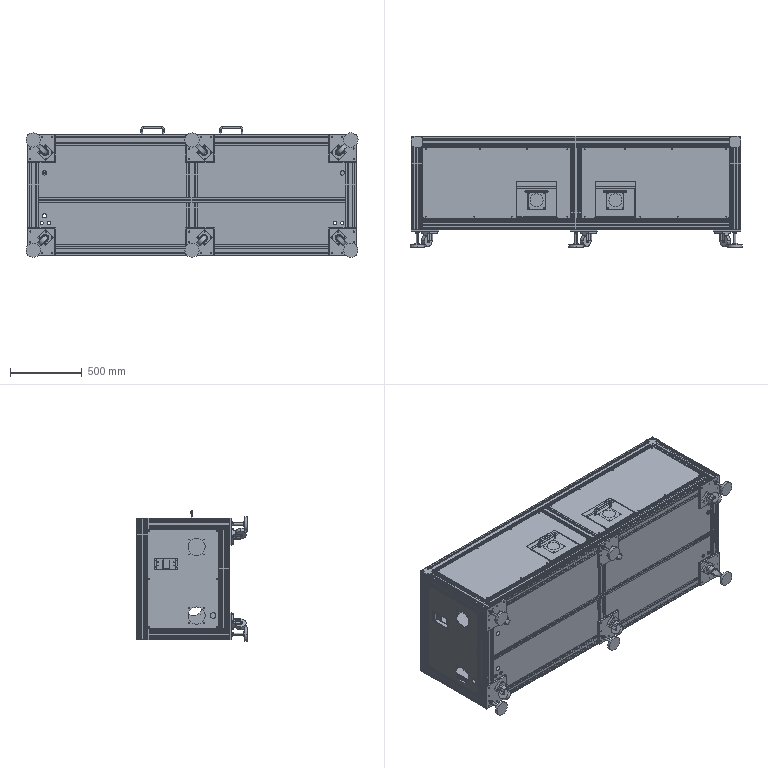Part | NX | 76 solids | 5191 faces | volume 65952723 mm3 | plane 3467 | cylinder 1486 | cone 170 | torus 56 | sphere 12 | commonest cylinder face diameters 2 x312 6.8 x180 7 x114 8 x108 11.8 x108 4 x84